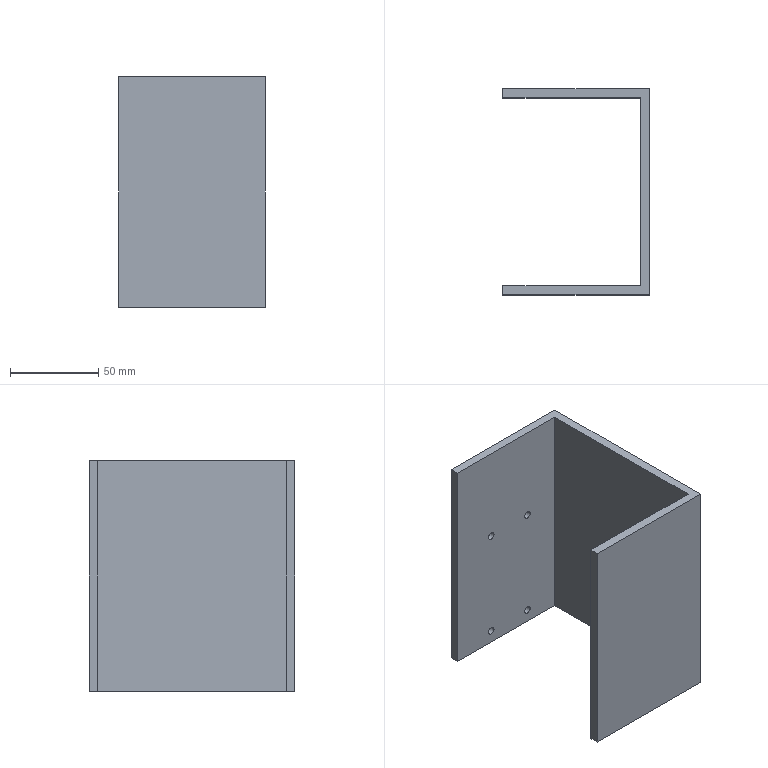Part | STEP file | Guide wheel mechanism revised.sldasm-Part-500 | 1 solid | 18 faces | box 83 x 117 x 131 mm | volume 178525 mm3 | plane 10 | cylinder 8 | commonest cylinder face diameters 4.3 x8
STEP:
#1=CARTESIAN_POINT('',(29.15,112.,8.4));
#2=VERTEX_POINT('',#1);
#3=CARTESIAN_POINT('',(24.85,112.,8.4));
#4=VERTEX_POINT('',#3);
#5=CARTESIAN_POINT('',(27.,112.,8.4));
#6=DIRECTION('',(0.,1.,0.));
#7=DIRECTION('',(1.,0.,0.));
#8=AXIS2_PLACEMENT_3D('',#5,#6,#7);
#9=CIRCLE('',#8,2.15);
#10=EDGE_CURVE('',#2,#4,#9,.T.);
#11=ORIENTED_EDGE('',*,*,#10,.F.);
#12=CARTESIAN_POINT('',(29.15,117.,8.4));
#13=VERTEX_POINT('',#12);
#14=CARTESIAN_POINT('',(29.15,-0.001,8.4));
#15=DIRECTION('',(0.,1.,0.));
#16=VECTOR('',#15,1000.);
#17=LINE('',#14,#16);
#18=EDGE_CURVE('',#2,#13,#17,.T.);
#19=ORIENTED_EDGE('',*,*,#18,.T.);
#20=CARTESIAN_POINT('',(24.85,117.,8.4));
#21=VERTEX_POINT('',#20);
#22=CARTESIAN_POINT('',(27.,117.,8.4));
#23=DIRECTION('',(0.,1.,0.));
#24=DIRECTION('',(-1.,0.,0.));
#25=AXIS2_PLACEMENT_3D('',#22,#23,#24);
#26=CIRCLE('',#25,2.15);
#27=EDGE_CURVE('',#13,#21,#26,.T.);
#28=ORIENTED_EDGE('',*,*,#27,.T.);
#29=CARTESIAN_POINT('',(24.85,-0.001,8.4));
#30=DIRECTION('',(0.,1.,0.));
#31=VECTOR('',#30,1000.);
#32=LINE('',#29,#31);
#33=EDGE_CURVE('',#4,#21,#32,.T.);
#34=ORIENTED_EDGE('',*,*,#33,.F.);
#35=EDGE_LOOP('',(#11,#19,#28,#34));
#36=FACE_OUTER_BOUND('',#35,.T.);
#37=CARTESIAN_POINT('',(27.,-0.001,8.4));
#38=DIRECTION('',(0.,1.,0.));
#39=DIRECTION('',(-1.,0.,0.));
#40=AXIS2_PLACEMENT_3D('',#37,#38,#39);
#41=CYLINDRICAL_SURFACE('',#40,2.15);
#42=ADVANCED_FACE('',(#36),#41,.F.);
#43=CARTESIAN_POINT('',(58.15,112.,8.4));
#44=VERTEX_POINT('',#43);
#45=CARTESIAN_POINT('',(53.85,112.,8.4));
#46=VERTEX_POINT('',#45);
#47=CARTESIAN_POINT('',(56.,112.,8.4));
#48=DIRECTION('',(0.,1.,0.));
#49=DIRECTION('',(1.,0.,0.));
#50=AXIS2_PLACEMENT_3D('',#47,#48,#49);
#51=CIRCLE('',#50,2.15);
#52=EDGE_CURVE('',#44,#46,#51,.T.);
#53=ORIENTED_EDGE('',*,*,#52,.F.);
#54=CARTESIAN_POINT('',(58.15,117.,8.4));
#55=VERTEX_POINT('',#54);
#56=CARTESIAN_POINT('',(58.15,-0.001,8.4));
#57=DIRECTION('',(0.,1.,0.));
#58=VECTOR('',#57,1000.);
#59=LINE('',#56,#58);
#60=EDGE_CURVE('',#44,#55,#59,.T.);
#61=ORIENTED_EDGE('',*,*,#60,.T.);
#62=CARTESIAN_POINT('',(53.85,117.,8.4));
#63=VERTEX_POINT('',#62);
#64=CARTESIAN_POINT('',(56.,117.,8.4));
#65=DIRECTION('',(0.,1.,0.));
#66=DIRECTION('',(-1.,0.,0.));
#67=AXIS2_PLACEMENT_3D('',#64,#65,#66);
#68=CIRCLE('',#67,2.15);
#69=EDGE_CURVE('',#55,#63,#68,.T.);
#70=ORIENTED_EDGE('',*,*,#69,.T.);
#71=CARTESIAN_POINT('',(53.85,-0.001,8.4));
#72=DIRECTION('',(0.,1.,0.));
#73=VECTOR('',#72,1000.);
#74=LINE('',#71,#73);
#75=EDGE_CURVE('',#46,#63,#74,.T.);
#76=ORIENTED_EDGE('',*,*,#75,.F.);
#77=EDGE_LOOP('',(#53,#61,#70,#76));
#78=FACE_OUTER_BOUND('',#77,.T.);
#79=CARTESIAN_POINT('',(56.,-0.001,8.4));
#80=DIRECTION('',(0.,1.,0.));
#81=DIRECTION('',(-1.,0.,0.));
#82=AXIS2_PLACEMENT_3D('',#79,#80,#81);
#83=CYLINDRICAL_SURFACE('',#82,2.15);
#84=ADVANCED_FACE('',(#78),#83,.F.);
#85=CARTESIAN_POINT('',(58.15,112.,-57.5));
#86=VERTEX_POINT('',#85);
#87=CARTESIAN_POINT('',(53.85,112.,-57.5));
#88=VERTEX_POINT('',#87);
#89=CARTESIAN_POINT('',(56.,112.,-57.5));
#90=DIRECTION('',(0.,1.,0.));
#91=DIRECTION('',(1.,0.,0.));
#92=AXIS2_PLACEMENT_3D('',#89,#90,#91);
#93=CIRCLE('',#92,2.15);
#94=EDGE_CURVE('',#86,#88,#93,.T.);
#95=ORIENTED_EDGE('',*,*,#94,.F.);
#96=CARTESIAN_POINT('',(58.15,117.,-57.5));
#97=VERTEX_POINT('',#96);
#98=CARTESIAN_POINT('',(58.15,-0.001,-57.5));
#99=DIRECTION('',(0.,1.,0.));
#100=VECTOR('',#99,1000.);
#101=LINE('',#98,#100);
#102=EDGE_CURVE('',#86,#97,#101,.T.);
#103=ORIENTED_EDGE('',*,*,#102,.T.);
#104=CARTESIAN_POINT('',(53.85,117.,-57.5));
#105=VERTEX_POINT('',#104);
#106=CARTESIAN_POINT('',(56.,117.,-57.5));
#107=DIRECTION('',(0.,1.,0.));
#108=DIRECTION('',(-1.,0.,0.));
#109=AXIS2_PLACEMENT_3D('',#106,#107,#108);
#110=CIRCLE('',#109,2.15);
#111=EDGE_CURVE('',#97,#105,#110,.T.);
#112=ORIENTED_EDGE('',*,*,#111,.T.);
#113=CARTESIAN_POINT('',(53.85,-0.001,-57.5));
#114=DIRECTION('',(0.,1.,0.));
#115=VECTOR('',#114,1000.);
#116=LINE('',#113,#115);
#117=EDGE_CURVE('',#88,#105,#116,.T.);
#118=ORIENTED_EDGE('',*,*,#117,.F.);
#119=EDGE_LOOP('',(#95,#103,#112,#118));
#120=FACE_OUTER_BOUND('',#119,.T.);
#121=CARTESIAN_POINT('',(56.,-0.001,-57.5));
#122=DIRECTION('',(0.,1.,0.));
#123=DIRECTION('',(-1.,0.,0.));
#124=AXIS2_PLACEMENT_3D('',#121,#122,#123);
#125=CYLINDRICAL_SURFACE('',#124,2.15);
#126=ADVANCED_FACE('',(#120),#125,.F.);
#127=CARTESIAN_POINT('',(29.15,112.,-57.5));
#128=VERTEX_POINT('',#127);
#129=CARTESIAN_POINT('',(24.85,112.,-57.5));
#130=VERTEX_POINT('',#129);
#131=CARTESIAN_POINT('',(27.,112.,-57.5));
#132=DIRECTION('',(0.,1.,0.));
#133=DIRECTION('',(1.,0.,0.));
#134=AXIS2_PLACEMENT_3D('',#131,#132,#133);
#135=CIRCLE('',#134,2.15);
#136=EDGE_CURVE('',#128,#130,#135,.T.);
#137=ORIENTED_EDGE('',*,*,#136,.F.);
#138=CARTESIAN_POINT('',(29.15,117.,-57.5));
#139=VERTEX_POINT('',#138);
#140=CARTESIAN_POINT('',(29.15,-0.001,-57.5));
#141=DIRECTION('',(0.,1.,0.));
#142=VECTOR('',#141,1000.);
#143=LINE('',#140,#142);
#144=EDGE_CURVE('',#128,#139,#143,.T.);
#145=ORIENTED_EDGE('',*,*,#144,.T.);
#146=CARTESIAN_POINT('',(24.85,117.,-57.5));
#147=VERTEX_POINT('',#146);
#148=CARTESIAN_POINT('',(27.,117.,-57.5));
#149=DIRECTION('',(0.,1.,0.));
#150=DIRECTION('',(-1.,0.,0.));
#151=AXIS2_PLACEMENT_3D('',#148,#149,#150);
#152=CIRCLE('',#151,2.15);
#153=EDGE_CURVE('',#139,#147,#152,.T.);
#154=ORIENTED_EDGE('',*,*,#153,.T.);
#155=CARTESIAN_POINT('',(24.85,-0.001,-57.5));
#156=DIRECTION('',(0.,1.,0.));
#157=VECTOR('',#156,1000.);
#158=LINE('',#155,#157);
#159=EDGE_CURVE('',#130,#147,#158,.T.);
#160=ORIENTED_EDGE('',*,*,#159,.F.);
#161=EDGE_LOOP('',(#137,#145,#154,#160));
#162=FACE_OUTER_BOUND('',#161,.T.);
#163=CARTESIAN_POINT('',(27.,-0.001,-57.5));
#164=DIRECTION('',(0.,1.,0.));
#165=DIRECTION('',(-1.,0.,0.));
#166=AXIS2_PLACEMENT_3D('',#163,#164,#165);
#167=CYLINDRICAL_SURFACE('',#166,2.15);
#168=ADVANCED_FACE('',(#162),#167,.F.);
#169=CARTESIAN_POINT('',(27.,117.,8.4));
#170=DIRECTION('',(0.,1.,0.));
#171=DIRECTION('',(-1.,0.,0.));
#172=AXIS2_PLACEMENT_3D('',#169,#170,#171);
#173=CIRCLE('',#172,2.15);
#174=EDGE_CURVE('',#21,#13,#173,.T.);
#175=ORIENTED_EDGE('',*,*,#174,.F.);
#176=ORIENTED_EDGE('',*,*,#27,.F.);
#177=EDGE_LOOP('',(#175,#176));
#178=FACE_BOUND('',#177,.T.);
#179=CARTESIAN_POINT('',(56.,117.,8.4));
#180=DIRECTION('',(0.,1.,0.));
#181=DIRECTION('',(-1.,0.,0.));
#182=AXIS2_PLACEMENT_3D('',#179,#180,#181);
#183=CIRCLE('',#182,2.15);
#184=EDGE_CURVE('',#63,#55,#183,.T.);
#185=ORIENTED_EDGE('',*,*,#184,.F.);
#186=ORIENTED_EDGE('',*,*,#69,.F.);
#187=EDGE_LOOP('',(#185,#186));
#188=FACE_BOUND('',#187,.T.);
#189=CARTESIAN_POINT('',(56.,117.,-57.5));
#190=DIRECTION('',(0.,1.,0.));
#191=DIRECTION('',(-1.,0.,0.));
#192=AXIS2_PLACEMENT_3D('',#189,#190,#191);
#193=CIRCLE('',#192,2.15);
#194=EDGE_CURVE('',#105,#97,#193,.T.);
#195=ORIENTED_EDGE('',*,*,#194,.F.);
#196=ORIENTED_EDGE('',*,*,#111,.F.);
#197=EDGE_LOOP('',(#195,#196));
#198=FACE_BOUND('',#197,.T.);
#199=CARTESIAN_POINT('',(27.,117.,-57.5));
#200=DIRECTION('',(0.,1.,0.));
#201=DIRECTION('',(-1.,0.,0.));
#202=AXIS2_PLACEMENT_3D('',#199,#200,#201);
#203=CIRCLE('',#202,2.15);
#204=EDGE_CURVE('',#147,#139,#203,.T.);
#205=ORIENTED_EDGE('',*,*,#204,.F.);
#206=ORIENTED_EDGE('',*,*,#153,.F.);
#207=EDGE_LOOP('',(#205,#206));
#208=FACE_BOUND('',#207,.T.);
#209=CARTESIAN_POINT('',(83.,117.,-65.5));
#210=VERTEX_POINT('',#209);
#211=CARTESIAN_POINT('',(0.,117.,-65.5));
#212=VERTEX_POINT('',#211);
#213=CARTESIAN_POINT('',(83.,117.,-65.5));
#214=DIRECTION('',(-1.,0.,0.));
#215=VECTOR('',#214,1000.);
#216=LINE('',#213,#215);
#217=EDGE_CURVE('',#210,#212,#216,.T.);
#218=ORIENTED_EDGE('',*,*,#217,.T.);
#219=CARTESIAN_POINT('',(0.,117.,65.5));
#220=VERTEX_POINT('',#219);
#221=CARTESIAN_POINT('',(0.,117.,65.5));
#222=DIRECTION('',(0.,0.,-1.));
#223=VECTOR('',#222,1000.);
#224=LINE('',#221,#223);
#225=EDGE_CURVE('',#220,#212,#224,.T.);
#226=ORIENTED_EDGE('',*,*,#225,.F.);
#227=CARTESIAN_POINT('',(83.,117.,65.5));
#228=VERTEX_POINT('',#227);
#229=CARTESIAN_POINT('',(83.,117.,65.5));
#230=DIRECTION('',(-1.,0.,0.));
#231=VECTOR('',#230,1000.);
#232=LINE('',#229,#231);
#233=EDGE_CURVE('',#228,#220,#232,.T.);
#234=ORIENTED_EDGE('',*,*,#233,.F.);
#235=CARTESIAN_POINT('',(83.,117.,65.5));
#236=DIRECTION('',(0.,0.,-1.));
#237=VECTOR('',#236,1000.);
#238=LINE('',#235,#237);
#239=EDGE_CURVE('',#228,#210,#238,.T.);
#240=ORIENTED_EDGE('',*,*,#239,.T.);
#241=EDGE_LOOP('',(#218,#226,#234,#240));
#242=FACE_OUTER_BOUND('',#241,.T.);
#243=CARTESIAN_POINT('',(83.,117.,65.5));
#244=DIRECTION('',(0.,-1.,0.));
#245=DIRECTION('',(1.,0.,0.));
#246=AXIS2_PLACEMENT_3D('',#243,#244,#245);
#247=PLANE('',#246);
#248=ADVANCED_FACE('',(#178,#188,#198,#208,#242),#247,.F.);
#249=CARTESIAN_POINT('',(0.,112.,-65.5));
#250=VERTEX_POINT('',#249);
#251=CARTESIAN_POINT('',(0.,112.,-65.5));
#252=DIRECTION('',(0.,1.,0.));
#253=VECTOR('',#252,1000.);
#254=LINE('',#251,#253);
#255=EDGE_CURVE('',#250,#212,#254,.T.);
#256=ORIENTED_EDGE('',*,*,#255,.F.);
#257=CARTESIAN_POINT('',(0.,112.,65.5));
#258=VERTEX_POINT('',#257);
#259=CARTESIAN_POINT('',(0.,112.,65.5));
#260=DIRECTION('',(0.,0.,-1.));
#261=VECTOR('',#260,1000.);
#262=LINE('',#259,#261);
#263=EDGE_CURVE('',#258,#250,#262,.T.);
#264=ORIENTED_EDGE('',*,*,#263,.F.);
#265=CARTESIAN_POINT('',(0.,112.,65.5));
#266=DIRECTION('',(0.,1.,0.));
#267=VECTOR('',#266,1000.);
#268=LINE('',#265,#267);
#269=EDGE_CURVE('',#258,#220,#268,.T.);
#270=ORIENTED_EDGE('',*,*,#269,.T.);
#271=ORIENTED_EDGE('',*,*,#225,.T.);
#272=EDGE_LOOP('',(#256,#264,#270,#271));
#273=FACE_OUTER_BOUND('',#272,.T.);
#274=CARTESIAN_POINT('',(0.,112.,65.5));
#275=DIRECTION('',(-1.,0.,0.));
#276=DIRECTION('',(0.,-1.,0.));
#277=AXIS2_PLACEMENT_3D('',#274,#275,#276);
#278=PLANE('',#277);
#279=ADVANCED_FACE('',(#273),#278,.T.);
#280=CARTESIAN_POINT('',(27.,112.,8.4));
#281=DIRECTION('',(0.,1.,0.));
#282=DIRECTION('',(1.,0.,0.));
#283=AXIS2_PLACEMENT_3D('',#280,#281,#282);
#284=CIRCLE('',#283,2.15);
#285=EDGE_CURVE('',#4,#2,#284,.T.);
#286=ORIENTED_EDGE('',*,*,#285,.T.);
#287=ORIENTED_EDGE('',*,*,#10,.T.);
#288=EDGE_LOOP('',(#286,#287));
#289=FACE_BOUND('',#288,.T.);
#290=CARTESIAN_POINT('',(56.,112.,8.4));
#291=DIRECTION('',(0.,1.,0.));
#292=DIRECTION('',(1.,0.,0.));
#293=AXIS2_PLACEMENT_3D('',#290,#291,#292);
#294=CIRCLE('',#293,2.15);
#295=EDGE_CURVE('',#46,#44,#294,.T.);
#296=ORIENTED_EDGE('',*,*,#295,.T.);
#297=ORIENTED_EDGE('',*,*,#52,.T.);
#298=EDGE_LOOP('',(#296,#297));
#299=FACE_BOUND('',#298,.T.);
#300=CARTESIAN_POINT('',(56.,112.,-57.5));
#301=DIRECTION('',(0.,1.,0.));
#302=DIRECTION('',(1.,0.,0.));
#303=AXIS2_PLACEMENT_3D('',#300,#301,#302);
#304=CIRCLE('',#303,2.15);
#305=EDGE_CURVE('',#88,#86,#304,.T.);
#306=ORIENTED_EDGE('',*,*,#305,.T.);
#307=ORIENTED_EDGE('',*,*,#94,.T.);
#308=EDGE_LOOP('',(#306,#307));
#309=FACE_BOUND('',#308,.T.);
#310=CARTESIAN_POINT('',(27.,112.,-57.5));
#311=DIRECTION('',(0.,1.,0.));
#312=DIRECTION('',(1.,0.,0.));
#313=AXIS2_PLACEMENT_3D('',#310,#311,#312);
#314=CIRCLE('',#313,2.15);
#315=EDGE_CURVE('',#130,#128,#314,.T.);
#316=ORIENTED_EDGE('',*,*,#315,.T.);
#317=ORIENTED_EDGE('',*,*,#136,.T.);
#318=EDGE_LOOP('',(#316,#317));
#319=FACE_BOUND('',#318,.T.);
#320=CARTESIAN_POINT('',(78.,112.,-65.5));
#321=VERTEX_POINT('',#320);
#322=CARTESIAN_POINT('',(83.,112.,-65.5));
#323=DIRECTION('',(-1.,0.,0.));
#324=VECTOR('',#323,1000.);
#325=LINE('',#322,#324);
#326=EDGE_CURVE('',#321,#250,#325,.T.);
#327=ORIENTED_EDGE('',*,*,#326,.F.);
#328=CARTESIAN_POINT('',(78.,112.,65.5));
#329=VERTEX_POINT('',#328);
#330=CARTESIAN_POINT('',(78.,112.,65.5));
#331=DIRECTION('',(0.,0.,-1.));
#332=VECTOR('',#331,1000.);
#333=LINE('',#330,#332);
#334=EDGE_CURVE('',#329,#321,#333,.T.);
#335=ORIENTED_EDGE('',*,*,#334,.F.);
#336=CARTESIAN_POINT('',(83.,112.,65.5));
#337=DIRECTION('',(-1.,0.,0.));
#338=VECTOR('',#337,1000.);
#339=LINE('',#336,#338);
#340=EDGE_CURVE('',#329,#258,#339,.T.);
#341=ORIENTED_EDGE('',*,*,#340,.T.);
#342=ORIENTED_EDGE('',*,*,#263,.T.);
#343=EDGE_LOOP('',(#327,#335,#341,#342));
#344=FACE_OUTER_BOUND('',#343,.T.);
#345=CARTESIAN_POINT('',(83.,112.,65.5));
#346=DIRECTION('',(0.,-1.,0.));
#347=DIRECTION('',(1.,0.,0.));
#348=AXIS2_PLACEMENT_3D('',#345,#346,#347);
#349=PLANE('',#348);
#350=ADVANCED_FACE('',(#289,#299,#309,#319,#344),#349,.T.);
#351=CARTESIAN_POINT('',(78.,5.,-65.5));
#352=VERTEX_POINT('',#351);
#353=CARTESIAN_POINT('',(78.,0.,-65.5));
#354=DIRECTION('',(0.,1.,0.));
#355=VECTOR('',#354,1000.);
#356=LINE('',#353,#355);
#357=EDGE_CURVE('',#352,#321,#356,.T.);
#358=ORIENTED_EDGE('',*,*,#357,.F.);
#359=CARTESIAN_POINT('',(78.,5.,65.5));
#360=VERTEX_POINT('',#359);
#361=CARTESIAN_POINT('',(78.,5.,65.5));
#362=DIRECTION('',(0.,0.,-1.));
#363=VECTOR('',#362,1000.);
#364=LINE('',#361,#363);
#365=EDGE_CURVE('',#360,#352,#364,.T.);
#366=ORIENTED_EDGE('',*,*,#365,.F.);
#367=CARTESIAN_POINT('',(78.,0.,65.5));
#368=DIRECTION('',(0.,1.,0.));
#369=VECTOR('',#368,1000.);
#370=LINE('',#367,#369);
#371=EDGE_CURVE('',#360,#329,#370,.T.);
#372=ORIENTED_EDGE('',*,*,#371,.T.);
#373=ORIENTED_EDGE('',*,*,#334,.T.);
#374=EDGE_LOOP('',(#358,#366,#372,#373));
#375=FACE_OUTER_BOUND('',#374,.T.);
#376=CARTESIAN_POINT('',(78.,0.,65.5));
#377=DIRECTION('',(-1.,0.,0.));
#378=DIRECTION('',(0.,0.,1.));
#379=AXIS2_PLACEMENT_3D('',#376,#377,#378);
#380=PLANE('',#379);
#381=ADVANCED_FACE('',(#375),#380,.T.);
#382=CARTESIAN_POINT('',(0.,5.,-65.5));
#383=VERTEX_POINT('',#382);
#384=CARTESIAN_POINT('',(0.,5.,-65.5));
#385=DIRECTION('',(1.,0.,0.));
#386=VECTOR('',#385,1000.);
#387=LINE('',#384,#386);
#388=EDGE_CURVE('',#383,#352,#387,.T.);
#389=ORIENTED_EDGE('',*,*,#388,.F.);
#390=CARTESIAN_POINT('',(0.,5.,65.5));
#391=VERTEX_POINT('',#390);
#392=CARTESIAN_POINT('',(0.,5.,65.5));
#393=DIRECTION('',(0.,0.,-1.));
#394=VECTOR('',#393,1000.);
#395=LINE('',#392,#394);
#396=EDGE_CURVE('',#391,#383,#395,.T.);
#397=ORIENTED_EDGE('',*,*,#396,.F.);
#398=CARTESIAN_POINT('',(0.,5.,65.5));
#399=DIRECTION('',(1.,0.,0.));
#400=VECTOR('',#399,1000.);
#401=LINE('',#398,#400);
#402=EDGE_CURVE('',#391,#360,#401,.T.);
#403=ORIENTED_EDGE('',*,*,#402,.T.);
#404=ORIENTED_EDGE('',*,*,#365,.T.);
#405=EDGE_LOOP('',(#389,#397,#403,#404));
#406=FACE_OUTER_BOUND('',#405,.T.);
#407=CARTESIAN_POINT('',(0.,5.,65.5));
#408=DIRECTION('',(0.,1.,0.));
#409=DIRECTION('',(0.,0.,1.));
#410=AXIS2_PLACEMENT_3D('',#407,#408,#409);
#411=PLANE('',#410);
#412=ADVANCED_FACE('',(#406),#411,.T.);
#413=CARTESIAN_POINT('',(0.,0.,-65.5));
#414=VERTEX_POINT('',#413);
#415=CARTESIAN_POINT('',(0.,0.,-65.5));
#416=DIRECTION('',(0.,1.,0.));
#417=VECTOR('',#416,1000.);
#418=LINE('',#415,#417);
#419=EDGE_CURVE('',#414,#383,#418,.T.);
#420=ORIENTED_EDGE('',*,*,#419,.F.);
#421=CARTESIAN_POINT('',(0.,0.,65.5));
#422=VERTEX_POINT('',#421);
#423=CARTESIAN_POINT('',(0.,0.,65.5));
#424=DIRECTION('',(0.,0.,-1.));
#425=VECTOR('',#424,1000.);
#426=LINE('',#423,#425);
#427=EDGE_CURVE('',#422,#414,#426,.T.);
#428=ORIENTED_EDGE('',*,*,#427,.F.);
#429=CARTESIAN_POINT('',(0.,0.,65.5));
#430=DIRECTION('',(0.,1.,0.));
#431=VECTOR('',#430,1000.);
#432=LINE('',#429,#431);
#433=EDGE_CURVE('',#422,#391,#432,.T.);
#434=ORIENTED_EDGE('',*,*,#433,.T.);
#435=ORIENTED_EDGE('',*,*,#396,.T.);
#436=EDGE_LOOP('',(#420,#428,#434,#435));
#437=FACE_OUTER_BOUND('',#436,.T.);
#438=CARTESIAN_POINT('',(0.,0.,65.5));
#439=DIRECTION('',(-1.,0.,0.));
#440=DIRECTION('',(0.,0.,1.));
#441=AXIS2_PLACEMENT_3D('',#438,#439,#440);
#442=PLANE('',#441);
#443=ADVANCED_FACE('',(#437),#442,.T.);
#444=CARTESIAN_POINT('',(83.,0.,-65.5));
#445=VERTEX_POINT('',#444);
#446=CARTESIAN_POINT('',(0.,0.,-65.5));
#447=DIRECTION('',(1.,0.,0.));
#448=VECTOR('',#447,1000.);
#449=LINE('',#446,#448);
#450=EDGE_CURVE('',#414,#445,#449,.T.);
#451=ORIENTED_EDGE('',*,*,#450,.T.);
#452=CARTESIAN_POINT('',(83.,0.,65.5));
#453=VERTEX_POINT('',#452);
#454=CARTESIAN_POINT('',(83.,0.,65.5));
#455=DIRECTION('',(0.,0.,-1.));
#456=VECTOR('',#455,1000.);
#457=LINE('',#454,#456);
#458=EDGE_CURVE('',#453,#445,#457,.T.);
#459=ORIENTED_EDGE('',*,*,#458,.F.);
#460=CARTESIAN_POINT('',(0.,0.,65.5));
#461=DIRECTION('',(1.,0.,0.));
#462=VECTOR('',#461,1000.);
#463=LINE('',#460,#462);
#464=EDGE_CURVE('',#422,#453,#463,.T.);
#465=ORIENTED_EDGE('',*,*,#464,.F.);
#466=ORIENTED_EDGE('',*,*,#427,.T.);
#467=EDGE_LOOP('',(#451,#459,#465,#466));
#468=FACE_OUTER_BOUND('',#467,.T.);
#469=CARTESIAN_POINT('',(0.,0.,65.5));
#470=DIRECTION('',(0.,1.,0.));
#471=DIRECTION('',(0.,0.,1.));
#472=AXIS2_PLACEMENT_3D('',#469,#470,#471);
#473=PLANE('',#472);
#474=ADVANCED_FACE('',(#468),#473,.F.);
#475=CARTESIAN_POINT('',(83.,0.,-65.5));
#476=DIRECTION('',(0.,1.,0.));
#477=VECTOR('',#476,1000.);
#478=LINE('',#475,#477);
#479=EDGE_CURVE('',#445,#210,#478,.T.);
#480=ORIENTED_EDGE('',*,*,#479,.T.);
#481=ORIENTED_EDGE('',*,*,#239,.F.);
#482=CARTESIAN_POINT('',(83.,0.,65.5));
#483=DIRECTION('',(0.,1.,0.));
#484=VECTOR('',#483,1000.);
#485=LINE('',#482,#484);
#486=EDGE_CURVE('',#453,#228,#485,.T.);
#487=ORIENTED_EDGE('',*,*,#486,.F.);
#488=ORIENTED_EDGE('',*,*,#458,.T.);
#489=EDGE_LOOP('',(#480,#481,#487,#488));
#490=FACE_OUTER_BOUND('',#489,.T.);
#491=CARTESIAN_POINT('',(83.,0.,65.5));
#492=DIRECTION('',(-1.,0.,0.));
#493=DIRECTION('',(0.,0.,1.));
#494=AXIS2_PLACEMENT_3D('',#491,#492,#493);
#495=PLANE('',#494);
#496=ADVANCED_FACE('',(#490),#495,.F.);
#497=ORIENTED_EDGE('',*,*,#233,.T.);
#498=ORIENTED_EDGE('',*,*,#269,.F.);
#499=ORIENTED_EDGE('',*,*,#340,.F.);
#500=ORIENTED_EDGE('',*,*,#371,.F.);
#501=ORIENTED_EDGE('',*,*,#402,.F.);
#502=ORIENTED_EDGE('',*,*,#433,.F.);
#503=ORIENTED_EDGE('',*,*,#464,.T.);
#504=ORIENTED_EDGE('',*,*,#486,.T.);
#505=EDGE_LOOP('',(#497,#498,#499,#500,#501,#502,#503,#504));
#506=FACE_OUTER_BOUND('',#505,.T.);
#507=CARTESIAN_POINT('',(0.,0.,65.5));
#508=DIRECTION('',(0.,0.,-1.));
#509=DIRECTION('',(-1.,0.,0.));
#510=AXIS2_PLACEMENT_3D('',#507,#508,#509);
#511=PLANE('',#510);
#512=ADVANCED_FACE('',(#506),#511,.F.);
#513=ORIENTED_EDGE('',*,*,#217,.F.);
#514=ORIENTED_EDGE('',*,*,#479,.F.);
#515=ORIENTED_EDGE('',*,*,#450,.F.);
#516=ORIENTED_EDGE('',*,*,#419,.T.);
#517=ORIENTED_EDGE('',*,*,#388,.T.);
#518=ORIENTED_EDGE('',*,*,#357,.T.);
#519=ORIENTED_EDGE('',*,*,#326,.T.);
#520=ORIENTED_EDGE('',*,*,#255,.T.);
#521=EDGE_LOOP('',(#513,#514,#515,#516,#517,#518,#519,#520));
#522=FACE_OUTER_BOUND('',#521,.T.);
#523=CARTESIAN_POINT('',(0.,0.,-65.5));
#524=DIRECTION('',(0.,0.,-1.));
#525=DIRECTION('',(-1.,0.,0.));
#526=AXIS2_PLACEMENT_3D('',#523,#524,#525);
#527=PLANE('',#526);
#528=ADVANCED_FACE('',(#522),#527,.T.);
#529=ORIENTED_EDGE('',*,*,#144,.F.);
#530=ORIENTED_EDGE('',*,*,#315,.F.);
#531=ORIENTED_EDGE('',*,*,#159,.T.);
#532=ORIENTED_EDGE('',*,*,#204,.T.);
#533=EDGE_LOOP('',(#529,#530,#531,#532));
#534=FACE_OUTER_BOUND('',#533,.T.);
#535=CARTESIAN_POINT('',(27.,-0.001,-57.5));
#536=DIRECTION('',(0.,1.,0.));
#537=DIRECTION('',(-1.,0.,0.));
#538=AXIS2_PLACEMENT_3D('',#535,#536,#537);
#539=CYLINDRICAL_SURFACE('',#538,2.15);
#540=ADVANCED_FACE('',(#534),#539,.F.);
#541=ORIENTED_EDGE('',*,*,#102,.F.);
#542=ORIENTED_EDGE('',*,*,#305,.F.);
#543=ORIENTED_EDGE('',*,*,#117,.T.);
#544=ORIENTED_EDGE('',*,*,#194,.T.);
#545=EDGE_LOOP('',(#541,#542,#543,#544));
#546=FACE_OUTER_BOUND('',#545,.T.);
#547=CARTESIAN_POINT('',(56.,-0.001,-57.5));
#548=DIRECTION('',(0.,1.,0.));
#549=DIRECTION('',(-1.,0.,0.));
#550=AXIS2_PLACEMENT_3D('',#547,#548,#549);
#551=CYLINDRICAL_SURFACE('',#550,2.15);
#552=ADVANCED_FACE('',(#546),#551,.F.);
#553=ORIENTED_EDGE('',*,*,#60,.F.);
#554=ORIENTED_EDGE('',*,*,#295,.F.);
#555=ORIENTED_EDGE('',*,*,#75,.T.);
#556=ORIENTED_EDGE('',*,*,#184,.T.);
#557=EDGE_LOOP('',(#553,#554,#555,#556));
#558=FACE_OUTER_BOUND('',#557,.T.);
#559=CARTESIAN_POINT('',(56.,-0.001,8.4));
#560=DIRECTION('',(0.,1.,0.));
#561=DIRECTION('',(-1.,0.,0.));
#562=AXIS2_PLACEMENT_3D('',#559,#560,#561);
#563=CYLINDRICAL_SURFACE('',#562,2.15);
#564=ADVANCED_FACE('',(#558),#563,.F.);
#565=ORIENTED_EDGE('',*,*,#18,.F.);
#566=ORIENTED_EDGE('',*,*,#285,.F.);
#567=ORIENTED_EDGE('',*,*,#33,.T.);
#568=ORIENTED_EDGE('',*,*,#174,.T.);
#569=EDGE_LOOP('',(#565,#566,#567,#568));
#570=FACE_OUTER_BOUND('',#569,.T.);
#571=CARTESIAN_POINT('',(27.,-0.001,8.4));
#572=DIRECTION('',(0.,1.,0.));
#573=DIRECTION('',(-1.,0.,0.));
#574=AXIS2_PLACEMENT_3D('',#571,#572,#573);
#575=CYLINDRICAL_SURFACE('',#574,2.15);
#576=ADVANCED_FACE('',(#570),#575,.F.);
#577=CLOSED_SHELL('',(#42,#84,#126,#168,#248,#279,#350,#381,#412,#443,#474,#496,#512,#528,#540,#552,#564,#576));
#578=MANIFOLD_SOLID_BREP('',#577);
#579=CARTESIAN_POINT('',(0.,0.,0.));
#580=DIRECTION('',(0.,0.,1.));
#581=DIRECTION('',(1.,0.,0.));
#582=AXIS2_PLACEMENT_3D('',#579,#580,#581);
#583=(LENGTH_UNIT()NAMED_UNIT(*)SI_UNIT(.MILLI.,.METRE.));
#584=UNCERTAINTY_MEASURE_WITH_UNIT(LENGTH_MEASURE(0.00001),#583,'','');
#585=(NAMED_UNIT(*)PLANE_ANGLE_UNIT()SI_UNIT($,.RADIAN.));
#586=(NAMED_UNIT(*)SI_UNIT($,.STERADIAN.)SOLID_ANGLE_UNIT());
#587=(GEOMETRIC_REPRESENTATION_CONTEXT(3)GLOBAL_UNCERTAINTY_ASSIGNED_CONTEXT((#584))GLOBAL_UNIT_ASSIGNED_CONTEXT((#583,#585,#586))REPRESENTATION_CONTEXT('',''));
#588=ADVANCED_BREP_SHAPE_REPRESENTATION('',(#578,#582),#587);